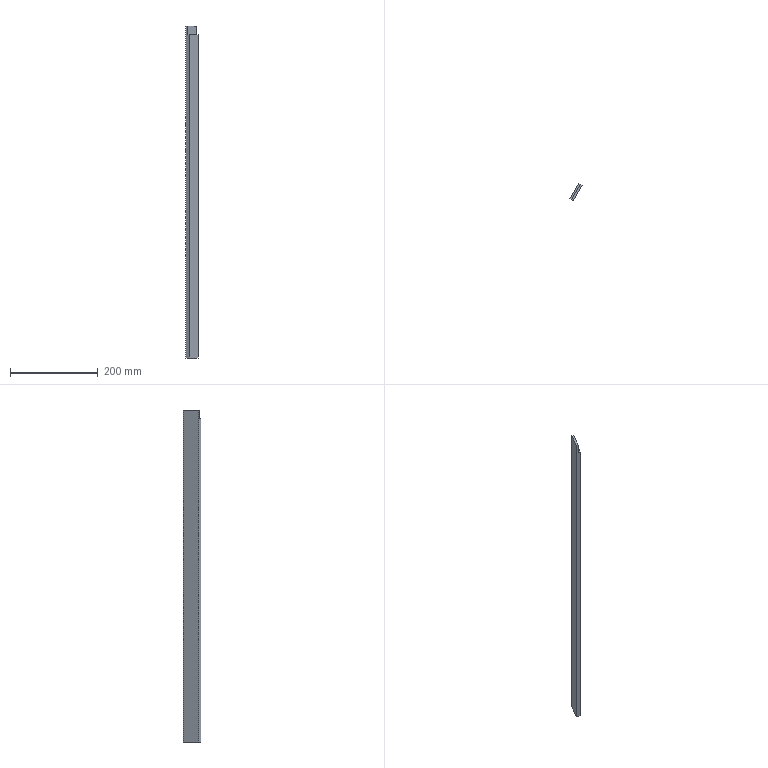Part | SolidWorks | features BaseBody 1 | 1 solid | 8 faces | box 27.565 x 39.009 x 756 mm | volume 260372 mm3 | plane 8
STEP:
#1=CARTESIAN_POINT('',(-207.873,1749.849,-387.));
#2=VERTEX_POINT('',#1);
#3=CARTESIAN_POINT('',(-187.873,1784.49,-387.));
#4=VERTEX_POINT('',#3);
#5=CARTESIAN_POINT('',(-197.873,1767.17,-387.));
#6=DIRECTION('',(0.5,0.866,0.));
#7=VECTOR('',#6,1000.);
#8=LINE('',#5,#7);
#9=EDGE_CURVE('',#2,#4,#8,.T.);
#10=ORIENTED_EDGE('',*,*,#9,.T.);
#11=CARTESIAN_POINT('',(-187.873,1784.49,-1143.));
#12=VERTEX_POINT('',#11);
#13=CARTESIAN_POINT('',(-187.873,1784.49,-543.));
#14=DIRECTION('',(0.,0.,-1.));
#15=VECTOR('',#14,1000.);
#16=LINE('',#13,#15);
#17=EDGE_CURVE('',#4,#12,#16,.T.);
#18=ORIENTED_EDGE('',*,*,#17,.T.);
#19=CARTESIAN_POINT('',(-207.873,1749.849,-1143.));
#20=VERTEX_POINT('',#19);
#21=CARTESIAN_POINT('',(-197.873,1767.17,-1143.));
#22=DIRECTION('',(-0.5,-0.866,0.));
#23=VECTOR('',#22,1000.);
#24=LINE('',#21,#23);
#25=EDGE_CURVE('',#12,#20,#24,.T.);
#26=ORIENTED_EDGE('',*,*,#25,.T.);
#27=CARTESIAN_POINT('',(-207.873,1749.849,-543.));
#28=DIRECTION('',(0.,0.,1.));
#29=VECTOR('',#28,1000.);
#30=LINE('',#27,#29);
#31=EDGE_CURVE('',#20,#2,#30,.T.);
#32=ORIENTED_EDGE('',*,*,#31,.T.);
#33=EDGE_LOOP('',(#10,#18,#26,#32));
#34=FACE_OUTER_BOUND('',#33,.T.);
#35=CARTESIAN_POINT('',(-197.873,1767.17,-543.));
#36=DIRECTION('',(-0.866,0.5,0.));
#37=DIRECTION('',(-0.5,-0.866,0.));
#38=AXIS2_PLACEMENT_3D('',#35,#36,#37);
#39=PLANE('',#38);
#40=ADVANCED_FACE('',(#34),#39,.T.);
#41=CARTESIAN_POINT('',(-180.308,1780.122,-1143.));
#42=VERTEX_POINT('',#41);
#43=CARTESIAN_POINT('',(-180.308,1780.122,-407.));
#44=VERTEX_POINT('',#43);
#45=CARTESIAN_POINT('',(-180.308,1780.122,-1143.));
#46=DIRECTION('',(0.,0.,1.));
#47=VECTOR('',#46,1000.);
#48=LINE('',#45,#47);
#49=EDGE_CURVE('',#42,#44,#48,.T.);
#50=ORIENTED_EDGE('',*,*,#49,.F.);
#51=CARTESIAN_POINT('',(-187.873,1784.49,-1143.));
#52=DIRECTION('',(0.866,-0.5,0.));
#53=VECTOR('',#52,1000.);
#54=LINE('',#51,#53);
#55=EDGE_CURVE('',#12,#42,#54,.T.);
#56=ORIENTED_EDGE('',*,*,#55,.F.);
#57=ORIENTED_EDGE('',*,*,#17,.F.);
#58=CARTESIAN_POINT('',(-184.409,1782.49,-387.));
#59=VERTEX_POINT('',#58);
#60=CARTESIAN_POINT('',(-187.873,1784.49,-387.));
#61=DIRECTION('',(-0.866,0.5,0.));
#62=VECTOR('',#61,1000.);
#63=LINE('',#60,#62);
#64=EDGE_CURVE('',#59,#4,#63,.T.);
#65=ORIENTED_EDGE('',*,*,#64,.F.);
#66=CARTESIAN_POINT('',(-184.409,1782.49,-407.));
#67=VERTEX_POINT('',#66);
#68=CARTESIAN_POINT('',(-184.409,1782.49,-1143.));
#69=DIRECTION('',(0.,0.,1.));
#70=VECTOR('',#69,1000.);
#71=LINE('',#68,#70);
#72=EDGE_CURVE('',#67,#59,#71,.T.);
#73=ORIENTED_EDGE('',*,*,#72,.F.);
#74=CARTESIAN_POINT('',(-187.873,1784.49,-407.));
#75=DIRECTION('',(-0.866,0.5,0.));
#76=VECTOR('',#75,1000.);
#77=LINE('',#74,#76);
#78=EDGE_CURVE('',#44,#67,#77,.T.);
#79=ORIENTED_EDGE('',*,*,#78,.F.);
#80=EDGE_LOOP('',(#50,#56,#57,#65,#73,#79));
#81=FACE_OUTER_BOUND('',#80,.T.);
#82=CARTESIAN_POINT('',(-187.873,1784.49,-1143.));
#83=DIRECTION('',(-0.5,-0.866,0.));
#84=DIRECTION('',(0.866,-0.5,0.));
#85=AXIS2_PLACEMENT_3D('',#82,#83,#84);
#86=PLANE('',#85);
#87=ADVANCED_FACE('',(#81),#86,.F.);
#88=ORIENTED_EDGE('',*,*,#9,.F.);
#89=CARTESIAN_POINT('',(-204.409,1747.849,-387.));
#90=VERTEX_POINT('',#89);
#91=CARTESIAN_POINT('',(-204.409,1747.849,-387.));
#92=DIRECTION('',(-0.866,0.5,0.));
#93=VECTOR('',#92,1000.);
#94=LINE('',#91,#93);
#95=EDGE_CURVE('',#90,#2,#94,.T.);
#96=ORIENTED_EDGE('',*,*,#95,.F.);
#97=CARTESIAN_POINT('',(-184.409,1782.49,-387.));
#98=DIRECTION('',(-0.5,-0.866,0.));
#99=VECTOR('',#98,1000.);
#100=LINE('',#97,#99);
#101=EDGE_CURVE('',#59,#90,#100,.T.);
#102=ORIENTED_EDGE('',*,*,#101,.F.);
#103=ORIENTED_EDGE('',*,*,#64,.T.);
#104=EDGE_LOOP('',(#88,#96,#102,#103));
#105=FACE_OUTER_BOUND('',#104,.T.);
#106=CARTESIAN_POINT('',(-207.873,1749.849,-387.));
#107=DIRECTION('',(0.,0.,-1.));
#108=DIRECTION('',(-1.,0.,0.));
#109=AXIS2_PLACEMENT_3D('',#106,#107,#108);
#110=PLANE('',#109);
#111=ADVANCED_FACE('',(#105),#110,.F.);
#112=CARTESIAN_POINT('',(-204.409,1747.849,-407.));
#113=VERTEX_POINT('',#112);
#114=CARTESIAN_POINT('',(-204.409,1747.849,-1143.));
#115=DIRECTION('',(0.,0.,-1.));
#116=VECTOR('',#115,1000.);
#117=LINE('',#114,#116);
#118=EDGE_CURVE('',#90,#113,#117,.T.);
#119=ORIENTED_EDGE('',*,*,#118,.F.);
#120=ORIENTED_EDGE('',*,*,#95,.T.);
#121=ORIENTED_EDGE('',*,*,#31,.F.);
#122=CARTESIAN_POINT('',(-200.308,1745.481,-1143.));
#123=VERTEX_POINT('',#122);
#124=CARTESIAN_POINT('',(-207.873,1749.849,-1143.));
#125=DIRECTION('',(-0.866,0.5,0.));
#126=VECTOR('',#125,1000.);
#127=LINE('',#124,#126);
#128=EDGE_CURVE('',#123,#20,#127,.T.);
#129=ORIENTED_EDGE('',*,*,#128,.F.);
#130=CARTESIAN_POINT('',(-200.308,1745.481,-407.));
#131=VERTEX_POINT('',#130);
#132=CARTESIAN_POINT('',(-200.308,1745.481,-1143.));
#133=DIRECTION('',(0.,0.,-1.));
#134=VECTOR('',#133,1000.);
#135=LINE('',#132,#134);
#136=EDGE_CURVE('',#131,#123,#135,.T.);
#137=ORIENTED_EDGE('',*,*,#136,.F.);
#138=CARTESIAN_POINT('',(-207.873,1749.849,-407.));
#139=DIRECTION('',(0.866,-0.5,0.));
#140=VECTOR('',#139,1000.);
#141=LINE('',#138,#140);
#142=EDGE_CURVE('',#113,#131,#141,.T.);
#143=ORIENTED_EDGE('',*,*,#142,.F.);
#144=EDGE_LOOP('',(#119,#120,#121,#129,#137,#143));
#145=FACE_OUTER_BOUND('',#144,.T.);
#146=CARTESIAN_POINT('',(-207.873,1749.849,-1143.));
#147=DIRECTION('',(0.5,0.866,0.));
#148=DIRECTION('',(-0.866,0.5,0.));
#149=AXIS2_PLACEMENT_3D('',#146,#147,#148);
#150=PLANE('',#149);
#151=ADVANCED_FACE('',(#145),#150,.F.);
#152=ORIENTED_EDGE('',*,*,#25,.F.);
#153=ORIENTED_EDGE('',*,*,#55,.T.);
#154=CARTESIAN_POINT('',(-200.308,1745.481,-1143.));
#155=DIRECTION('',(0.5,0.866,0.));
#156=VECTOR('',#155,1000.);
#157=LINE('',#154,#156);
#158=EDGE_CURVE('',#123,#42,#157,.T.);
#159=ORIENTED_EDGE('',*,*,#158,.F.);
#160=ORIENTED_EDGE('',*,*,#128,.T.);
#161=EDGE_LOOP('',(#152,#153,#159,#160));
#162=FACE_OUTER_BOUND('',#161,.T.);
#163=CARTESIAN_POINT('',(-207.873,1749.849,-1143.));
#164=DIRECTION('',(0.,0.,1.));
#165=DIRECTION('',(1.,0.,0.));
#166=AXIS2_PLACEMENT_3D('',#163,#164,#165);
#167=PLANE('',#166);
#168=ADVANCED_FACE('',(#162),#167,.F.);
#169=CARTESIAN_POINT('',(-204.409,1747.849,-407.));
#170=DIRECTION('',(0.5,0.866,0.));
#171=VECTOR('',#170,1000.);
#172=LINE('',#169,#171);
#173=EDGE_CURVE('',#113,#67,#172,.T.);
#174=ORIENTED_EDGE('',*,*,#173,.F.);
#175=ORIENTED_EDGE('',*,*,#142,.T.);
#176=CARTESIAN_POINT('',(-180.308,1780.122,-407.));
#177=DIRECTION('',(-0.5,-0.866,0.));
#178=VECTOR('',#177,1000.);
#179=LINE('',#176,#178);
#180=EDGE_CURVE('',#44,#131,#179,.T.);
#181=ORIENTED_EDGE('',*,*,#180,.F.);
#182=ORIENTED_EDGE('',*,*,#78,.T.);
#183=EDGE_LOOP('',(#174,#175,#181,#182));
#184=FACE_OUTER_BOUND('',#183,.T.);
#185=CARTESIAN_POINT('',(-204.409,1747.849,-407.));
#186=DIRECTION('',(0.,0.,-1.));
#187=DIRECTION('',(-1.,0.,0.));
#188=AXIS2_PLACEMENT_3D('',#185,#186,#187);
#189=PLANE('',#188);
#190=ADVANCED_FACE('',(#184),#189,.F.);
#191=ORIENTED_EDGE('',*,*,#136,.T.);
#192=ORIENTED_EDGE('',*,*,#158,.T.);
#193=ORIENTED_EDGE('',*,*,#49,.T.);
#194=ORIENTED_EDGE('',*,*,#180,.T.);
#195=EDGE_LOOP('',(#191,#192,#193,#194));
#196=FACE_OUTER_BOUND('',#195,.T.);
#197=CARTESIAN_POINT('',(-190.308,1762.802,-543.));
#198=DIRECTION('',(-0.866,0.5,0.));
#199=DIRECTION('',(-0.5,-0.866,0.));
#200=AXIS2_PLACEMENT_3D('',#197,#198,#199);
#201=PLANE('',#200);
#202=ADVANCED_FACE('',(#196),#201,.F.);
#203=ORIENTED_EDGE('',*,*,#101,.T.);
#204=ORIENTED_EDGE('',*,*,#118,.T.);
#205=ORIENTED_EDGE('',*,*,#173,.T.);
#206=ORIENTED_EDGE('',*,*,#72,.T.);
#207=EDGE_LOOP('',(#203,#204,#205,#206));
#208=FACE_OUTER_BOUND('',#207,.T.);
#209=CARTESIAN_POINT('',(-194.409,1765.17,-387.));
#210=DIRECTION('',(0.866,-0.5,0.));
#211=DIRECTION('',(0.5,0.866,0.));
#212=AXIS2_PLACEMENT_3D('',#209,#210,#211);
#213=PLANE('',#212);
#214=ADVANCED_FACE('',(#208),#213,.T.);
#215=CLOSED_SHELL('',(#40,#87,#111,#151,#168,#190,#202,#214));
#216=MANIFOLD_SOLID_BREP('',#215);
#217=CARTESIAN_POINT('',(0.,0.,0.));
#218=DIRECTION('',(0.,0.,1.));
#219=DIRECTION('',(1.,0.,0.));
#220=AXIS2_PLACEMENT_3D('',#217,#218,#219);
#221=(LENGTH_UNIT()NAMED_UNIT(*)SI_UNIT(.MILLI.,.METRE.));
#222=UNCERTAINTY_MEASURE_WITH_UNIT(LENGTH_MEASURE(0.00001),#221,'','');
#223=(NAMED_UNIT(*)PLANE_ANGLE_UNIT()SI_UNIT($,.RADIAN.));
#224=(NAMED_UNIT(*)SI_UNIT($,.STERADIAN.)SOLID_ANGLE_UNIT());
#225=(GEOMETRIC_REPRESENTATION_CONTEXT(3)GLOBAL_UNCERTAINTY_ASSIGNED_CONTEXT((#222))GLOBAL_UNIT_ASSIGNED_CONTEXT((#221,#223,#224))REPRESENTATION_CONTEXT('',''));
#226=ADVANCED_BREP_SHAPE_REPRESENTATION('',(#216,#220),#225);